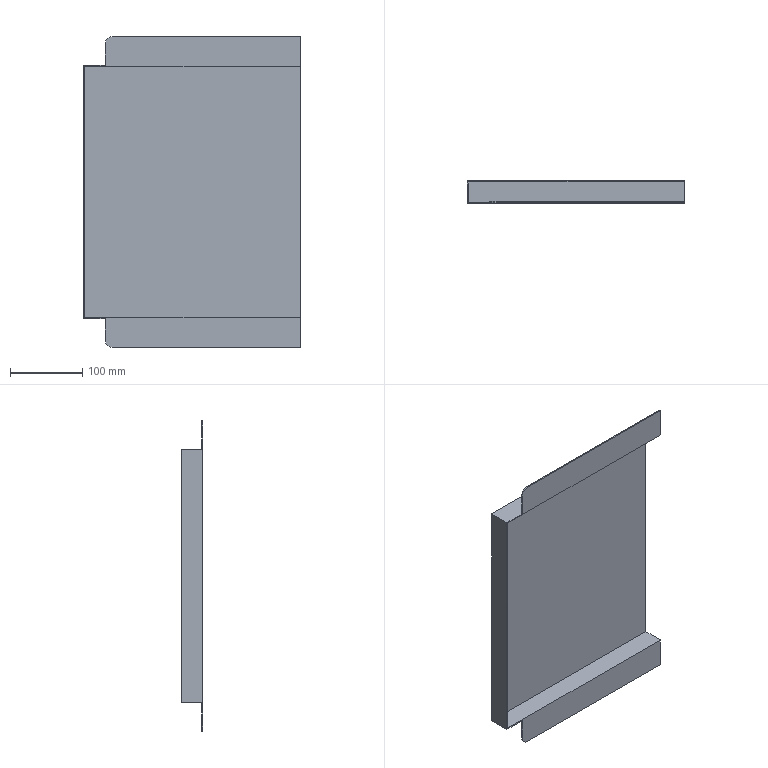Part | STEP file | B-BAN5_1-2 | 1 solid | 18 faces | box 300 x 30 x 430 mm | volume 230320 mm3 | plane 16 | cylinder 2 | commonest cylinder face diameters 20 x2
STEP:
#1=CARTESIAN_POINT('',(100.,30.,-175.));
#2=VERTEX_POINT('',#1);
#3=CARTESIAN_POINT('',(100.,30.,175.));
#4=VERTEX_POINT('',#3);
#5=CARTESIAN_POINT('',(100.,30.,0.));
#6=DIRECTION('',(0.,0.,1.));
#7=VECTOR('',#6,1000.);
#8=LINE('',#5,#7);
#9=EDGE_CURVE('',#2,#4,#8,.T.);
#10=ORIENTED_EDGE('',*,*,#9,.F.);
#11=CARTESIAN_POINT('',(-200.,30.,-175.));
#12=VERTEX_POINT('',#11);
#13=CARTESIAN_POINT('',(0.,30.,-175.));
#14=DIRECTION('',(-1.,0.,0.));
#15=VECTOR('',#14,1000.);
#16=LINE('',#13,#15);
#17=EDGE_CURVE('',#2,#12,#16,.T.);
#18=ORIENTED_EDGE('',*,*,#17,.T.);
#19=CARTESIAN_POINT('',(-200.,30.,175.));
#20=VERTEX_POINT('',#19);
#21=CARTESIAN_POINT('',(-200.,30.,0.));
#22=DIRECTION('',(0.,0.,1.));
#23=VECTOR('',#22,1000.);
#24=LINE('',#21,#23);
#25=EDGE_CURVE('',#12,#20,#24,.T.);
#26=ORIENTED_EDGE('',*,*,#25,.T.);
#27=CARTESIAN_POINT('',(0.,30.,175.));
#28=DIRECTION('',(1.,0.,0.));
#29=VECTOR('',#28,1000.);
#30=LINE('',#27,#29);
#31=EDGE_CURVE('',#20,#4,#30,.T.);
#32=ORIENTED_EDGE('',*,*,#31,.T.);
#33=EDGE_LOOP('',(#10,#18,#26,#32));
#34=FACE_OUTER_BOUND('',#33,.T.);
#35=CARTESIAN_POINT('',(0.,30.,0.));
#36=DIRECTION('',(0.,1.,0.));
#37=DIRECTION('',(0.,0.,1.));
#38=AXIS2_PLACEMENT_3D('',#35,#36,#37);
#39=PLANE('',#38);
#40=ADVANCED_FACE('',(#34),#39,.T.);
#41=CARTESIAN_POINT('',(-200.,0.,-175.));
#42=VERTEX_POINT('',#41);
#43=CARTESIAN_POINT('',(-200.,0.,-175.));
#44=DIRECTION('',(0.,-1.,0.));
#45=VECTOR('',#44,1000.);
#46=LINE('',#43,#45);
#47=EDGE_CURVE('',#12,#42,#46,.T.);
#48=ORIENTED_EDGE('',*,*,#47,.T.);
#49=CARTESIAN_POINT('',(-200.,0.,175.));
#50=VERTEX_POINT('',#49);
#51=CARTESIAN_POINT('',(-200.,0.,-175.));
#52=DIRECTION('',(0.,0.,1.));
#53=VECTOR('',#52,1000.);
#54=LINE('',#51,#53);
#55=EDGE_CURVE('',#42,#50,#54,.T.);
#56=ORIENTED_EDGE('',*,*,#55,.T.);
#57=CARTESIAN_POINT('',(-200.,0.,175.));
#58=DIRECTION('',(0.,1.,0.));
#59=VECTOR('',#58,1000.);
#60=LINE('',#57,#59);
#61=EDGE_CURVE('',#50,#20,#60,.T.);
#62=ORIENTED_EDGE('',*,*,#61,.T.);
#63=ORIENTED_EDGE('',*,*,#25,.F.);
#64=EDGE_LOOP('',(#48,#56,#62,#63));
#65=FACE_OUTER_BOUND('',#64,.T.);
#66=CARTESIAN_POINT('',(-200.,0.,-175.));
#67=DIRECTION('',(-1.,0.,0.));
#68=DIRECTION('',(0.,0.,1.));
#69=AXIS2_PLACEMENT_3D('',#66,#67,#68);
#70=PLANE('',#69);
#71=ADVANCED_FACE('',(#65),#70,.T.);
#72=CARTESIAN_POINT('',(100.,1.5,-175.));
#73=VERTEX_POINT('',#72);
#74=CARTESIAN_POINT('',(100.,0.,-175.));
#75=DIRECTION('',(0.,1.,0.));
#76=VECTOR('',#75,1000.);
#77=LINE('',#74,#76);
#78=EDGE_CURVE('',#73,#2,#77,.T.);
#79=ORIENTED_EDGE('',*,*,#78,.F.);
#80=CARTESIAN_POINT('',(-170.,1.5,-175.));
#81=VERTEX_POINT('',#80);
#82=CARTESIAN_POINT('',(200.,1.5,-175.));
#83=DIRECTION('',(-1.,0.,0.));
#84=VECTOR('',#83,1000.);
#85=LINE('',#82,#84);
#86=EDGE_CURVE('',#73,#81,#85,.T.);
#87=ORIENTED_EDGE('',*,*,#86,.T.);
#88=CARTESIAN_POINT('',(-170.,0.,-175.));
#89=VERTEX_POINT('',#88);
#90=CARTESIAN_POINT('',(-170.,0.,-175.));
#91=DIRECTION('',(0.,1.,0.));
#92=VECTOR('',#91,1000.);
#93=LINE('',#90,#92);
#94=EDGE_CURVE('',#89,#81,#93,.T.);
#95=ORIENTED_EDGE('',*,*,#94,.F.);
#96=CARTESIAN_POINT('',(200.,0.,-175.));
#97=DIRECTION('',(-1.,0.,0.));
#98=VECTOR('',#97,1000.);
#99=LINE('',#96,#98);
#100=EDGE_CURVE('',#89,#42,#99,.T.);
#101=ORIENTED_EDGE('',*,*,#100,.T.);
#102=ORIENTED_EDGE('',*,*,#47,.F.);
#103=ORIENTED_EDGE('',*,*,#17,.F.);
#104=EDGE_LOOP('',(#79,#87,#95,#101,#102,#103));
#105=FACE_OUTER_BOUND('',#104,.T.);
#106=CARTESIAN_POINT('',(200.,0.,-175.));
#107=DIRECTION('',(0.,0.,-1.));
#108=DIRECTION('',(-1.,0.,0.));
#109=AXIS2_PLACEMENT_3D('',#106,#107,#108);
#110=PLANE('',#109);
#111=ADVANCED_FACE('',(#105),#110,.T.);
#112=CARTESIAN_POINT('',(100.,1.5,175.));
#113=VERTEX_POINT('',#112);
#114=CARTESIAN_POINT('',(100.,0.,175.));
#115=DIRECTION('',(0.,-1.,0.));
#116=VECTOR('',#115,1000.);
#117=LINE('',#114,#116);
#118=EDGE_CURVE('',#4,#113,#117,.T.);
#119=ORIENTED_EDGE('',*,*,#118,.F.);
#120=ORIENTED_EDGE('',*,*,#31,.F.);
#121=ORIENTED_EDGE('',*,*,#61,.F.);
#122=CARTESIAN_POINT('',(-170.,0.,175.));
#123=VERTEX_POINT('',#122);
#124=CARTESIAN_POINT('',(-200.,0.,175.));
#125=DIRECTION('',(1.,0.,0.));
#126=VECTOR('',#125,1000.);
#127=LINE('',#124,#126);
#128=EDGE_CURVE('',#50,#123,#127,.T.);
#129=ORIENTED_EDGE('',*,*,#128,.T.);
#130=CARTESIAN_POINT('',(-170.,1.5,175.));
#131=VERTEX_POINT('',#130);
#132=CARTESIAN_POINT('',(-170.,0.,175.));
#133=DIRECTION('',(0.,-1.,0.));
#134=VECTOR('',#133,1000.);
#135=LINE('',#132,#134);
#136=EDGE_CURVE('',#131,#123,#135,.T.);
#137=ORIENTED_EDGE('',*,*,#136,.F.);
#138=CARTESIAN_POINT('',(-200.,1.5,175.));
#139=DIRECTION('',(1.,0.,0.));
#140=VECTOR('',#139,1000.);
#141=LINE('',#138,#140);
#142=EDGE_CURVE('',#131,#113,#141,.T.);
#143=ORIENTED_EDGE('',*,*,#142,.T.);
#144=EDGE_LOOP('',(#119,#120,#121,#129,#137,#143));
#145=FACE_OUTER_BOUND('',#144,.T.);
#146=CARTESIAN_POINT('',(-200.,0.,175.));
#147=DIRECTION('',(0.,0.,1.));
#148=DIRECTION('',(1.,0.,0.));
#149=AXIS2_PLACEMENT_3D('',#146,#147,#148);
#150=PLANE('',#149);
#151=ADVANCED_FACE('',(#145),#150,.T.);
#152=CARTESIAN_POINT('',(100.,0.,-215.));
#153=VERTEX_POINT('',#152);
#154=CARTESIAN_POINT('',(-160.,0.,-215.));
#155=VERTEX_POINT('',#154);
#156=CARTESIAN_POINT('',(0.,0.,-215.));
#157=DIRECTION('',(-1.,0.,0.));
#158=VECTOR('',#157,1000.);
#159=LINE('',#156,#158);
#160=EDGE_CURVE('',#153,#155,#159,.T.);
#161=ORIENTED_EDGE('',*,*,#160,.F.);
#162=CARTESIAN_POINT('',(100.,0.,-173.5));
#163=VERTEX_POINT('',#162);
#164=CARTESIAN_POINT('',(100.,0.,0.));
#165=DIRECTION('',(0.,0.,1.));
#166=VECTOR('',#165,1000.);
#167=LINE('',#164,#166);
#168=EDGE_CURVE('',#153,#163,#167,.T.);
#169=ORIENTED_EDGE('',*,*,#168,.T.);
#170=CARTESIAN_POINT('',(-198.5,0.,-173.5));
#171=VERTEX_POINT('',#170);
#172=CARTESIAN_POINT('',(0.,0.,-173.5));
#173=DIRECTION('',(1.,0.,0.));
#174=VECTOR('',#173,1000.);
#175=LINE('',#172,#174);
#176=EDGE_CURVE('',#171,#163,#175,.T.);
#177=ORIENTED_EDGE('',*,*,#176,.F.);
#178=CARTESIAN_POINT('',(-198.5,0.,173.5));
#179=VERTEX_POINT('',#178);
#180=CARTESIAN_POINT('',(-198.5,0.,0.));
#181=DIRECTION('',(0.,0.,-1.));
#182=VECTOR('',#181,1000.);
#183=LINE('',#180,#182);
#184=EDGE_CURVE('',#179,#171,#183,.T.);
#185=ORIENTED_EDGE('',*,*,#184,.F.);
#186=CARTESIAN_POINT('',(100.,0.,173.5));
#187=VERTEX_POINT('',#186);
#188=CARTESIAN_POINT('',(0.,0.,173.5));
#189=DIRECTION('',(-1.,0.,0.));
#190=VECTOR('',#189,1000.);
#191=LINE('',#188,#190);
#192=EDGE_CURVE('',#187,#179,#191,.T.);
#193=ORIENTED_EDGE('',*,*,#192,.F.);
#194=CARTESIAN_POINT('',(100.,0.,215.));
#195=VERTEX_POINT('',#194);
#196=CARTESIAN_POINT('',(100.,0.,0.));
#197=DIRECTION('',(0.,0.,1.));
#198=VECTOR('',#197,1000.);
#199=LINE('',#196,#198);
#200=EDGE_CURVE('',#187,#195,#199,.T.);
#201=ORIENTED_EDGE('',*,*,#200,.T.);
#202=CARTESIAN_POINT('',(-160.,0.,215.));
#203=VERTEX_POINT('',#202);
#204=CARTESIAN_POINT('',(0.,0.,215.));
#205=DIRECTION('',(1.,0.,0.));
#206=VECTOR('',#205,1000.);
#207=LINE('',#204,#206);
#208=EDGE_CURVE('',#203,#195,#207,.T.);
#209=ORIENTED_EDGE('',*,*,#208,.F.);
#210=CARTESIAN_POINT('',(-170.,0.,205.));
#211=VERTEX_POINT('',#210);
#212=CARTESIAN_POINT('',(-160.,0.,205.));
#213=DIRECTION('',(0.,1.,0.));
#214=DIRECTION('',(0.,0.,1.));
#215=AXIS2_PLACEMENT_3D('',#212,#213,#214);
#216=CIRCLE('',#215,10.);
#217=EDGE_CURVE('',#211,#203,#216,.T.);
#218=ORIENTED_EDGE('',*,*,#217,.F.);
#219=CARTESIAN_POINT('',(-170.,0.,0.));
#220=DIRECTION('',(0.,0.,1.));
#221=VECTOR('',#220,1000.);
#222=LINE('',#219,#221);
#223=EDGE_CURVE('',#123,#211,#222,.T.);
#224=ORIENTED_EDGE('',*,*,#223,.F.);
#225=ORIENTED_EDGE('',*,*,#128,.F.);
#226=ORIENTED_EDGE('',*,*,#55,.F.);
#227=ORIENTED_EDGE('',*,*,#100,.F.);
#228=CARTESIAN_POINT('',(-170.,0.,-205.));
#229=VERTEX_POINT('',#228);
#230=CARTESIAN_POINT('',(-170.,0.,0.));
#231=DIRECTION('',(0.,0.,1.));
#232=VECTOR('',#231,1000.);
#233=LINE('',#230,#232);
#234=EDGE_CURVE('',#229,#89,#233,.T.);
#235=ORIENTED_EDGE('',*,*,#234,.F.);
#236=CARTESIAN_POINT('',(-160.,0.,-205.));
#237=DIRECTION('',(0.,1.,0.));
#238=DIRECTION('',(0.,0.,1.));
#239=AXIS2_PLACEMENT_3D('',#236,#237,#238);
#240=CIRCLE('',#239,10.);
#241=EDGE_CURVE('',#155,#229,#240,.T.);
#242=ORIENTED_EDGE('',*,*,#241,.F.);
#243=EDGE_LOOP('',(#161,#169,#177,#185,#193,#201,#209,#218,#224,#225,#226,#227,#235,#242));
#244=FACE_OUTER_BOUND('',#243,.T.);
#245=CARTESIAN_POINT('',(0.,0.,0.));
#246=DIRECTION('',(0.,1.,0.));
#247=DIRECTION('',(0.,0.,1.));
#248=AXIS2_PLACEMENT_3D('',#245,#246,#247);
#249=PLANE('',#248);
#250=ADVANCED_FACE('',(#244),#249,.F.);
#251=ORIENTED_EDGE('',*,*,#86,.F.);
#252=CARTESIAN_POINT('',(100.,1.5,-215.));
#253=VERTEX_POINT('',#252);
#254=CARTESIAN_POINT('',(100.,1.5,0.));
#255=DIRECTION('',(0.,0.,-1.));
#256=VECTOR('',#255,1000.);
#257=LINE('',#254,#256);
#258=EDGE_CURVE('',#73,#253,#257,.T.);
#259=ORIENTED_EDGE('',*,*,#258,.T.);
#260=CARTESIAN_POINT('',(-160.,1.5,-215.));
#261=VERTEX_POINT('',#260);
#262=CARTESIAN_POINT('',(0.,1.5,-215.));
#263=DIRECTION('',(1.,0.,0.));
#264=VECTOR('',#263,1000.);
#265=LINE('',#262,#264);
#266=EDGE_CURVE('',#261,#253,#265,.T.);
#267=ORIENTED_EDGE('',*,*,#266,.F.);
#268=CARTESIAN_POINT('',(-170.,1.5,-205.));
#269=VERTEX_POINT('',#268);
#270=CARTESIAN_POINT('',(-160.,1.5,-205.));
#271=DIRECTION('',(0.,-1.,0.));
#272=DIRECTION('',(0.,0.,1.));
#273=AXIS2_PLACEMENT_3D('',#270,#271,#272);
#274=CIRCLE('',#273,10.);
#275=EDGE_CURVE('',#269,#261,#274,.T.);
#276=ORIENTED_EDGE('',*,*,#275,.F.);
#277=CARTESIAN_POINT('',(-170.,1.5,0.));
#278=DIRECTION('',(0.,0.,-1.));
#279=VECTOR('',#278,1000.);
#280=LINE('',#277,#279);
#281=EDGE_CURVE('',#81,#269,#280,.T.);
#282=ORIENTED_EDGE('',*,*,#281,.F.);
#283=EDGE_LOOP('',(#251,#259,#267,#276,#282));
#284=FACE_OUTER_BOUND('',#283,.T.);
#285=CARTESIAN_POINT('',(0.,1.5,0.));
#286=DIRECTION('',(0.,-1.,0.));
#287=DIRECTION('',(0.,0.,-1.));
#288=AXIS2_PLACEMENT_3D('',#285,#286,#287);
#289=PLANE('',#288);
#290=ADVANCED_FACE('',(#284),#289,.F.);
#291=ORIENTED_EDGE('',*,*,#176,.T.);
#292=CARTESIAN_POINT('',(100.,28.5,-173.5));
#293=VERTEX_POINT('',#292);
#294=CARTESIAN_POINT('',(100.,0.,-173.5));
#295=DIRECTION('',(0.,1.,0.));
#296=VECTOR('',#295,1000.);
#297=LINE('',#294,#296);
#298=EDGE_CURVE('',#163,#293,#297,.T.);
#299=ORIENTED_EDGE('',*,*,#298,.T.);
#300=CARTESIAN_POINT('',(-198.5,28.5,-173.5));
#301=VERTEX_POINT('',#300);
#302=CARTESIAN_POINT('',(200.,28.5,-173.5));
#303=DIRECTION('',(1.,0.,0.));
#304=VECTOR('',#303,1000.);
#305=LINE('',#302,#304);
#306=EDGE_CURVE('',#301,#293,#305,.T.);
#307=ORIENTED_EDGE('',*,*,#306,.F.);
#308=CARTESIAN_POINT('',(-198.5,0.,-173.5));
#309=DIRECTION('',(0.,1.,0.));
#310=VECTOR('',#309,1000.);
#311=LINE('',#308,#310);
#312=EDGE_CURVE('',#171,#301,#311,.T.);
#313=ORIENTED_EDGE('',*,*,#312,.F.);
#314=EDGE_LOOP('',(#291,#299,#307,#313));
#315=FACE_OUTER_BOUND('',#314,.T.);
#316=CARTESIAN_POINT('',(200.,0.,-173.5));
#317=DIRECTION('',(0.,0.,-1.));
#318=DIRECTION('',(-1.,0.,0.));
#319=AXIS2_PLACEMENT_3D('',#316,#317,#318);
#320=PLANE('',#319);
#321=ADVANCED_FACE('',(#315),#320,.F.);
#322=ORIENTED_EDGE('',*,*,#306,.T.);
#323=CARTESIAN_POINT('',(100.,28.5,173.5));
#324=VERTEX_POINT('',#323);
#325=CARTESIAN_POINT('',(100.,28.5,0.));
#326=DIRECTION('',(0.,0.,1.));
#327=VECTOR('',#326,1000.);
#328=LINE('',#325,#327);
#329=EDGE_CURVE('',#293,#324,#328,.T.);
#330=ORIENTED_EDGE('',*,*,#329,.T.);
#331=CARTESIAN_POINT('',(-198.5,28.5,173.5));
#332=VERTEX_POINT('',#331);
#333=CARTESIAN_POINT('',(0.,28.5,173.5));
#334=DIRECTION('',(1.,0.,0.));
#335=VECTOR('',#334,1000.);
#336=LINE('',#333,#335);
#337=EDGE_CURVE('',#332,#324,#336,.T.);
#338=ORIENTED_EDGE('',*,*,#337,.F.);
#339=CARTESIAN_POINT('',(-198.5,28.5,0.));
#340=DIRECTION('',(0.,0.,1.));
#341=VECTOR('',#340,1000.);
#342=LINE('',#339,#341);
#343=EDGE_CURVE('',#301,#332,#342,.T.);
#344=ORIENTED_EDGE('',*,*,#343,.F.);
#345=EDGE_LOOP('',(#322,#330,#338,#344));
#346=FACE_OUTER_BOUND('',#345,.T.);
#347=CARTESIAN_POINT('',(0.,28.5,0.));
#348=DIRECTION('',(0.,1.,0.));
#349=DIRECTION('',(0.,0.,1.));
#350=AXIS2_PLACEMENT_3D('',#347,#348,#349);
#351=PLANE('',#350);
#352=ADVANCED_FACE('',(#346),#351,.F.);
#353=ORIENTED_EDGE('',*,*,#337,.T.);
#354=CARTESIAN_POINT('',(100.,0.,173.5));
#355=DIRECTION('',(0.,-1.,0.));
#356=VECTOR('',#355,1000.);
#357=LINE('',#354,#356);
#358=EDGE_CURVE('',#324,#187,#357,.T.);
#359=ORIENTED_EDGE('',*,*,#358,.T.);
#360=ORIENTED_EDGE('',*,*,#192,.T.);
#361=CARTESIAN_POINT('',(-198.5,0.,173.5));
#362=DIRECTION('',(0.,-1.,0.));
#363=VECTOR('',#362,1000.);
#364=LINE('',#361,#363);
#365=EDGE_CURVE('',#332,#179,#364,.T.);
#366=ORIENTED_EDGE('',*,*,#365,.F.);
#367=EDGE_LOOP('',(#353,#359,#360,#366));
#368=FACE_OUTER_BOUND('',#367,.T.);
#369=CARTESIAN_POINT('',(-200.,0.,173.5));
#370=DIRECTION('',(0.,0.,1.));
#371=DIRECTION('',(1.,0.,0.));
#372=AXIS2_PLACEMENT_3D('',#369,#370,#371);
#373=PLANE('',#372);
#374=ADVANCED_FACE('',(#368),#373,.F.);
#375=CARTESIAN_POINT('',(100.,1.5,215.));
#376=VERTEX_POINT('',#375);
#377=CARTESIAN_POINT('',(-160.,1.5,215.));
#378=VERTEX_POINT('',#377);
#379=CARTESIAN_POINT('',(0.,1.5,215.));
#380=DIRECTION('',(-1.,0.,0.));
#381=VECTOR('',#380,1000.);
#382=LINE('',#379,#381);
#383=EDGE_CURVE('',#376,#378,#382,.T.);
#384=ORIENTED_EDGE('',*,*,#383,.F.);
#385=CARTESIAN_POINT('',(100.,1.5,0.));
#386=DIRECTION('',(0.,0.,-1.));
#387=VECTOR('',#386,1000.);
#388=LINE('',#385,#387);
#389=EDGE_CURVE('',#376,#113,#388,.T.);
#390=ORIENTED_EDGE('',*,*,#389,.T.);
#391=ORIENTED_EDGE('',*,*,#142,.F.);
#392=CARTESIAN_POINT('',(-170.,1.5,205.));
#393=VERTEX_POINT('',#392);
#394=CARTESIAN_POINT('',(-170.,1.5,0.));
#395=DIRECTION('',(0.,0.,-1.));
#396=VECTOR('',#395,1000.);
#397=LINE('',#394,#396);
#398=EDGE_CURVE('',#393,#131,#397,.T.);
#399=ORIENTED_EDGE('',*,*,#398,.F.);
#400=CARTESIAN_POINT('',(-160.,1.5,205.));
#401=DIRECTION('',(0.,-1.,0.));
#402=DIRECTION('',(0.,0.,1.));
#403=AXIS2_PLACEMENT_3D('',#400,#401,#402);
#404=CIRCLE('',#403,10.);
#405=EDGE_CURVE('',#378,#393,#404,.T.);
#406=ORIENTED_EDGE('',*,*,#405,.F.);
#407=EDGE_LOOP('',(#384,#390,#391,#399,#406));
#408=FACE_OUTER_BOUND('',#407,.T.);
#409=CARTESIAN_POINT('',(0.,1.5,0.));
#410=DIRECTION('',(0.,-1.,0.));
#411=DIRECTION('',(0.,0.,-1.));
#412=AXIS2_PLACEMENT_3D('',#409,#410,#411);
#413=PLANE('',#412);
#414=ADVANCED_FACE('',(#408),#413,.F.);
#415=CARTESIAN_POINT('',(100.,0.,-215.));
#416=DIRECTION('',(0.,1.,0.));
#417=VECTOR('',#416,1000.);
#418=LINE('',#415,#417);
#419=EDGE_CURVE('',#153,#253,#418,.T.);
#420=ORIENTED_EDGE('',*,*,#419,.F.);
#421=ORIENTED_EDGE('',*,*,#160,.T.);
#422=CARTESIAN_POINT('',(-160.,0.,-215.));
#423=DIRECTION('',(0.,1.,0.));
#424=VECTOR('',#423,1000.);
#425=LINE('',#422,#424);
#426=EDGE_CURVE('',#155,#261,#425,.T.);
#427=ORIENTED_EDGE('',*,*,#426,.T.);
#428=ORIENTED_EDGE('',*,*,#266,.T.);
#429=EDGE_LOOP('',(#420,#421,#427,#428));
#430=FACE_OUTER_BOUND('',#429,.T.);
#431=CARTESIAN_POINT('',(-170.,0.,-215.));
#432=DIRECTION('',(0.,0.,-1.));
#433=DIRECTION('',(-1.,0.,0.));
#434=AXIS2_PLACEMENT_3D('',#431,#432,#433);
#435=PLANE('',#434);
#436=ADVANCED_FACE('',(#430),#435,.T.);
#437=ORIENTED_EDGE('',*,*,#343,.T.);
#438=ORIENTED_EDGE('',*,*,#365,.T.);
#439=ORIENTED_EDGE('',*,*,#184,.T.);
#440=ORIENTED_EDGE('',*,*,#312,.T.);
#441=EDGE_LOOP('',(#437,#438,#439,#440));
#442=FACE_OUTER_BOUND('',#441,.T.);
#443=CARTESIAN_POINT('',(-198.5,0.,-175.));
#444=DIRECTION('',(-1.,0.,0.));
#445=DIRECTION('',(0.,0.,1.));
#446=AXIS2_PLACEMENT_3D('',#443,#444,#445);
#447=PLANE('',#446);
#448=ADVANCED_FACE('',(#442),#447,.F.);
#449=CARTESIAN_POINT('',(100.,0.,215.));
#450=DIRECTION('',(0.,-1.,0.));
#451=VECTOR('',#450,1000.);
#452=LINE('',#449,#451);
#453=EDGE_CURVE('',#376,#195,#452,.T.);
#454=ORIENTED_EDGE('',*,*,#453,.F.);
#455=ORIENTED_EDGE('',*,*,#383,.T.);
#456=CARTESIAN_POINT('',(-160.,0.,215.));
#457=DIRECTION('',(0.,-1.,0.));
#458=VECTOR('',#457,1000.);
#459=LINE('',#456,#458);
#460=EDGE_CURVE('',#378,#203,#459,.T.);
#461=ORIENTED_EDGE('',*,*,#460,.T.);
#462=ORIENTED_EDGE('',*,*,#208,.T.);
#463=EDGE_LOOP('',(#454,#455,#461,#462));
#464=FACE_OUTER_BOUND('',#463,.T.);
#465=CARTESIAN_POINT('',(200.,0.,215.));
#466=DIRECTION('',(0.,0.,1.));
#467=DIRECTION('',(1.,0.,0.));
#468=AXIS2_PLACEMENT_3D('',#465,#466,#467);
#469=PLANE('',#468);
#470=ADVANCED_FACE('',(#464),#469,.T.);
#471=ORIENTED_EDGE('',*,*,#460,.F.);
#472=ORIENTED_EDGE('',*,*,#405,.T.);
#473=CARTESIAN_POINT('',(-170.,-39.108,205.));
#474=DIRECTION('',(0.,-1.,0.));
#475=VECTOR('',#474,1000.);
#476=LINE('',#473,#475);
#477=EDGE_CURVE('',#393,#211,#476,.T.);
#478=ORIENTED_EDGE('',*,*,#477,.T.);
#479=ORIENTED_EDGE('',*,*,#217,.T.);
#480=EDGE_LOOP('',(#471,#472,#478,#479));
#481=FACE_OUTER_BOUND('',#480,.T.);
#482=CARTESIAN_POINT('',(-160.,-39.108,205.));
#483=DIRECTION('',(0.,1.,0.));
#484=DIRECTION('',(0.,0.,1.));
#485=AXIS2_PLACEMENT_3D('',#482,#483,#484);
#486=CYLINDRICAL_SURFACE('',#485,10.);
#487=ADVANCED_FACE('',(#481),#486,.T.);
#488=ORIENTED_EDGE('',*,*,#223,.T.);
#489=ORIENTED_EDGE('',*,*,#477,.F.);
#490=ORIENTED_EDGE('',*,*,#398,.T.);
#491=ORIENTED_EDGE('',*,*,#136,.T.);
#492=EDGE_LOOP('',(#488,#489,#490,#491));
#493=FACE_OUTER_BOUND('',#492,.T.);
#494=CARTESIAN_POINT('',(-170.,0.,215.));
#495=DIRECTION('',(-1.,0.,0.));
#496=DIRECTION('',(0.,0.,1.));
#497=AXIS2_PLACEMENT_3D('',#494,#495,#496);
#498=PLANE('',#497);
#499=ADVANCED_FACE('',(#493),#498,.T.);
#500=ORIENTED_EDGE('',*,*,#281,.T.);
#501=CARTESIAN_POINT('',(-170.,0.,-205.));
#502=DIRECTION('',(0.,-1.,0.));
#503=VECTOR('',#502,1000.);
#504=LINE('',#501,#503);
#505=EDGE_CURVE('',#269,#229,#504,.T.);
#506=ORIENTED_EDGE('',*,*,#505,.T.);
#507=ORIENTED_EDGE('',*,*,#234,.T.);
#508=ORIENTED_EDGE('',*,*,#94,.T.);
#509=EDGE_LOOP('',(#500,#506,#507,#508));
#510=FACE_OUTER_BOUND('',#509,.T.);
#511=CARTESIAN_POINT('',(-170.,0.,-175.));
#512=DIRECTION('',(-1.,0.,0.));
#513=DIRECTION('',(0.,0.,1.));
#514=AXIS2_PLACEMENT_3D('',#511,#512,#513);
#515=PLANE('',#514);
#516=ADVANCED_FACE('',(#510),#515,.T.);
#517=ORIENTED_EDGE('',*,*,#505,.F.);
#518=ORIENTED_EDGE('',*,*,#275,.T.);
#519=ORIENTED_EDGE('',*,*,#426,.F.);
#520=ORIENTED_EDGE('',*,*,#241,.T.);
#521=EDGE_LOOP('',(#517,#518,#519,#520));
#522=FACE_OUTER_BOUND('',#521,.T.);
#523=CARTESIAN_POINT('',(-160.,-39.108,-205.));
#524=DIRECTION('',(0.,1.,0.));
#525=DIRECTION('',(0.,0.,1.));
#526=AXIS2_PLACEMENT_3D('',#523,#524,#525);
#527=CYLINDRICAL_SURFACE('',#526,10.);
#528=ADVANCED_FACE('',(#522),#527,.T.);
#529=ORIENTED_EDGE('',*,*,#118,.T.);
#530=ORIENTED_EDGE('',*,*,#389,.F.);
#531=ORIENTED_EDGE('',*,*,#453,.T.);
#532=ORIENTED_EDGE('',*,*,#200,.F.);
#533=ORIENTED_EDGE('',*,*,#358,.F.);
#534=ORIENTED_EDGE('',*,*,#329,.F.);
#535=ORIENTED_EDGE('',*,*,#298,.F.);
#536=ORIENTED_EDGE('',*,*,#168,.F.);
#537=ORIENTED_EDGE('',*,*,#419,.T.);
#538=ORIENTED_EDGE('',*,*,#258,.F.);
#539=ORIENTED_EDGE('',*,*,#78,.T.);
#540=ORIENTED_EDGE('',*,*,#9,.T.);
#541=EDGE_LOOP('',(#529,#530,#531,#532,#533,#534,#535,#536,#537,#538,#539,#540));
#542=FACE_OUTER_BOUND('',#541,.T.);
#543=CARTESIAN_POINT('',(100.,-0.0001031,232.548));
#544=DIRECTION('',(-1.,0.,0.));
#545=DIRECTION('',(0.,0.,1.));
#546=AXIS2_PLACEMENT_3D('',#543,#544,#545);
#547=PLANE('',#546);
#548=ADVANCED_FACE('',(#542),#547,.F.);
#549=CLOSED_SHELL('',(#40,#71,#111,#151,#250,#290,#321,#352,#374,#414,#436,#448,#470,#487,#499,#516,#528,#548));
#550=MANIFOLD_SOLID_BREP('',#549);
#551=CARTESIAN_POINT('',(0.,0.,0.));
#552=DIRECTION('',(0.,0.,1.));
#553=DIRECTION('',(1.,0.,0.));
#554=AXIS2_PLACEMENT_3D('',#551,#552,#553);
#555=(LENGTH_UNIT()NAMED_UNIT(*)SI_UNIT(.MILLI.,.METRE.));
#556=UNCERTAINTY_MEASURE_WITH_UNIT(LENGTH_MEASURE(0.00001),#555,'','');
#557=(NAMED_UNIT(*)PLANE_ANGLE_UNIT()SI_UNIT($,.RADIAN.));
#558=(NAMED_UNIT(*)SI_UNIT($,.STERADIAN.)SOLID_ANGLE_UNIT());
#559=(GEOMETRIC_REPRESENTATION_CONTEXT(3)GLOBAL_UNCERTAINTY_ASSIGNED_CONTEXT((#556))GLOBAL_UNIT_ASSIGNED_CONTEXT((#555,#557,#558))REPRESENTATION_CONTEXT('',''));
#560=ADVANCED_BREP_SHAPE_REPRESENTATION('',(#550,#554),#559);